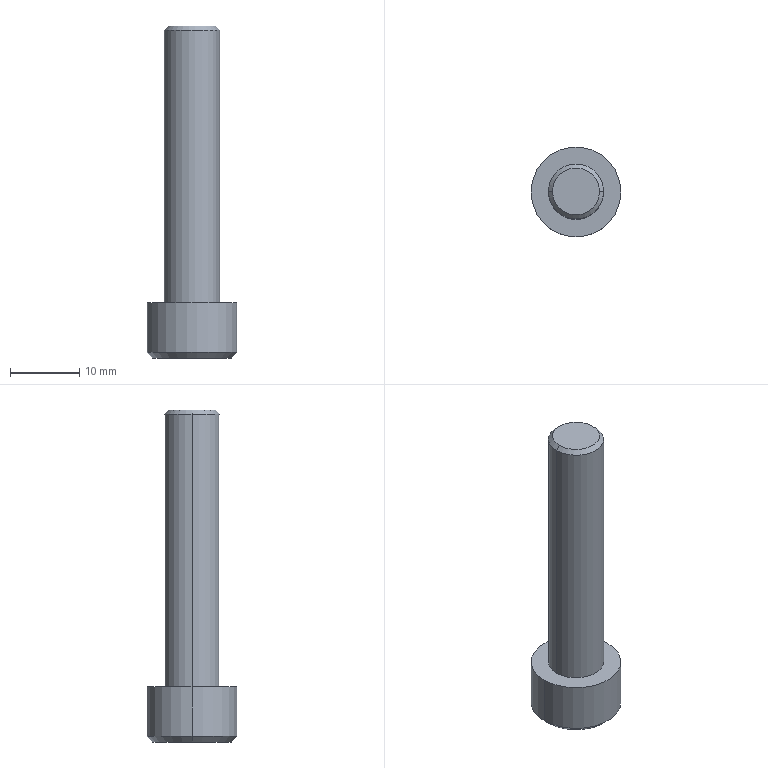Part | Creo | 1 solid | 18 faces | box 13 x 13 x 48 mm | volume 2906 mm3 | plane 10 | cylinder 4 | cone 4 | commonest cylinder face diameters 8 x2 13 x2
STEP:
#1=CARTESIAN_POINT('',(48.5,0.,-326.5));
#2=VERTEX_POINT('',#1);
#3=CARTESIAN_POINT('',(61.5,0.,-326.5));
#4=VERTEX_POINT('',#3);
#5=CARTESIAN_POINT('',(55.,0.,-326.5));
#6=DIRECTION('',(0.,0.,1.));
#7=DIRECTION('',(-1.,0.,0.));
#8=AXIS2_PLACEMENT_3D('',#5,#6,#7);
#9=CIRCLE('',#8,6.5);
#10=EDGE_CURVE('',#2,#4,#9,.T.);
#11=ORIENTED_EDGE('',*,*,#10,.F.);
#12=CARTESIAN_POINT('',(55.,0.,-326.5));
#13=DIRECTION('',(0.,0.,1.));
#14=DIRECTION('',(1.,0.,0.));
#15=AXIS2_PLACEMENT_3D('',#12,#13,#14);
#16=CIRCLE('',#15,6.5);
#17=EDGE_CURVE('',#4,#2,#16,.T.);
#18=ORIENTED_EDGE('',*,*,#17,.F.);
#19=EDGE_LOOP('',(#11,#18));
#20=FACE_OUTER_BOUND('',#19,.F.);
#21=CARTESIAN_POINT('',(59.,0.,-326.5));
#22=VERTEX_POINT('',#21);
#23=CARTESIAN_POINT('',(51.,0.,-326.5));
#24=VERTEX_POINT('',#23);
#25=CARTESIAN_POINT('',(55.,0.,-326.5));
#26=DIRECTION('',(0.,0.,-1.));
#27=DIRECTION('',(1.,0.,0.));
#28=AXIS2_PLACEMENT_3D('',#25,#26,#27);
#29=CIRCLE('',#28,4.);
#30=EDGE_CURVE('',#22,#24,#29,.T.);
#31=ORIENTED_EDGE('',*,*,#30,.F.);
#32=CARTESIAN_POINT('',(55.,0.,-326.5));
#33=DIRECTION('',(0.,0.,-1.));
#34=DIRECTION('',(-1.,0.,0.));
#35=AXIS2_PLACEMENT_3D('',#32,#33,#34);
#36=CIRCLE('',#35,4.);
#37=EDGE_CURVE('',#24,#22,#36,.T.);
#38=ORIENTED_EDGE('',*,*,#37,.F.);
#39=EDGE_LOOP('',(#31,#38));
#40=FACE_BOUND('',#39,.F.);
#41=CARTESIAN_POINT('',(55.,0.,-326.5));
#42=DIRECTION('',(0.,0.,1.));
#43=DIRECTION('',(1.,0.,0.));
#44=AXIS2_PLACEMENT_3D('',#41,#42,#43);
#45=PLANE('',#44);
#46=ADVANCED_FACE('',(#20,#40),#45,.T.);
#47=CARTESIAN_POINT('',(51.,0.,-287.1));
#48=VERTEX_POINT('',#47);
#49=CARTESIAN_POINT('',(59.,0.,-287.1));
#50=VERTEX_POINT('',#49);
#51=CARTESIAN_POINT('',(55.,0.,-287.1));
#52=DIRECTION('',(0.,0.,1.));
#53=DIRECTION('',(-1.,0.,0.));
#54=AXIS2_PLACEMENT_3D('',#51,#52,#53);
#55=CIRCLE('',#54,4.);
#56=EDGE_CURVE('',#48,#50,#55,.T.);
#57=ORIENTED_EDGE('',*,*,#56,.T.);
#58=CARTESIAN_POINT('',(59.,0.,-326.5));
#59=DIRECTION('',(0.,0.,1.));
#60=VECTOR('',#59,39.4);
#61=LINE('',#58,#60);
#62=EDGE_CURVE('',#22,#50,#61,.T.);
#63=ORIENTED_EDGE('',*,*,#62,.F.);
#64=ORIENTED_EDGE('',*,*,#30,.T.);
#65=CARTESIAN_POINT('',(51.,0.,-326.5));
#66=DIRECTION('',(0.,0.,1.));
#67=VECTOR('',#66,39.4);
#68=LINE('',#65,#67);
#69=EDGE_CURVE('',#24,#48,#68,.T.);
#70=ORIENTED_EDGE('',*,*,#69,.T.);
#71=EDGE_LOOP('',(#57,#63,#64,#70));
#72=FACE_OUTER_BOUND('',#71,.F.);
#73=CARTESIAN_POINT('',(55.,0.,-335.5));
#74=DIRECTION('',(0.,0.,1.));
#75=DIRECTION('',(1.,0.,0.));
#76=AXIS2_PLACEMENT_3D('',#73,#74,#75);
#77=CYLINDRICAL_SURFACE('',#76,4.);
#78=ADVANCED_FACE('',(#72),#77,.T.);
#79=CARTESIAN_POINT('',(51.6,0.,-286.5));
#80=VERTEX_POINT('',#79);
#81=CARTESIAN_POINT('',(58.4,0.,-286.5));
#82=VERTEX_POINT('',#81);
#83=CARTESIAN_POINT('',(55.,0.,-286.5));
#84=DIRECTION('',(0.,0.,1.));
#85=DIRECTION('',(-1.,0.,0.));
#86=AXIS2_PLACEMENT_3D('',#83,#84,#85);
#87=CIRCLE('',#86,3.4);
#88=EDGE_CURVE('',#80,#82,#87,.T.);
#89=ORIENTED_EDGE('',*,*,#88,.T.);
#90=CARTESIAN_POINT('',(58.4,0.,-286.5));
#91=DIRECTION('',(0.7071,0.,-0.7071));
#92=VECTOR('',#91,0.8485);
#93=LINE('',#90,#92);
#94=EDGE_CURVE('',#82,#50,#93,.T.);
#95=ORIENTED_EDGE('',*,*,#94,.T.);
#96=ORIENTED_EDGE('',*,*,#56,.F.);
#97=CARTESIAN_POINT('',(51.6,0.,-286.5));
#98=DIRECTION('',(-0.7071,0.,-0.7071));
#99=VECTOR('',#98,0.8485);
#100=LINE('',#97,#99);
#101=EDGE_CURVE('',#80,#48,#100,.T.);
#102=ORIENTED_EDGE('',*,*,#101,.F.);
#103=EDGE_LOOP('',(#89,#95,#96,#102));
#104=FACE_OUTER_BOUND('',#103,.F.);
#105=CARTESIAN_POINT('',(55.,0.,-286.8));
#106=DIRECTION('',(0.,0.,-1.));
#107=DIRECTION('',(-1.,0.,0.));
#108=AXIS2_PLACEMENT_3D('',#105,#106,#107);
#109=CONICAL_SURFACE('',#108,3.7,45.);
#110=ADVANCED_FACE('',(#104),#109,.T.);
#111=CARTESIAN_POINT('',(55.,0.,-286.5));
#112=DIRECTION('',(0.,0.,1.));
#113=DIRECTION('',(1.,0.,0.));
#114=AXIS2_PLACEMENT_3D('',#111,#112,#113);
#115=CIRCLE('',#114,3.4);
#116=EDGE_CURVE('',#82,#80,#115,.T.);
#117=ORIENTED_EDGE('',*,*,#116,.F.);
#118=ORIENTED_EDGE('',*,*,#88,.F.);
#119=EDGE_LOOP('',(#117,#118));
#120=FACE_OUTER_BOUND('',#119,.F.);
#121=CARTESIAN_POINT('',(55.,0.,-286.5));
#122=DIRECTION('',(0.,0.,1.));
#123=DIRECTION('',(1.,0.,0.));
#124=AXIS2_PLACEMENT_3D('',#121,#122,#123);
#125=PLANE('',#124);
#126=ADVANCED_FACE('',(#120),#125,.T.);
#127=ORIENTED_EDGE('',*,*,#116,.T.);
#128=ORIENTED_EDGE('',*,*,#101,.T.);
#129=CARTESIAN_POINT('',(55.,0.,-287.1));
#130=DIRECTION('',(0.,0.,1.));
#131=DIRECTION('',(1.,0.,0.));
#132=AXIS2_PLACEMENT_3D('',#129,#130,#131);
#133=CIRCLE('',#132,4.);
#134=EDGE_CURVE('',#50,#48,#133,.T.);
#135=ORIENTED_EDGE('',*,*,#134,.F.);
#136=ORIENTED_EDGE('',*,*,#94,.F.);
#137=EDGE_LOOP('',(#127,#128,#135,#136));
#138=FACE_OUTER_BOUND('',#137,.F.);
#139=CARTESIAN_POINT('',(55.,0.,-286.8));
#140=DIRECTION('',(0.,0.,-1.));
#141=DIRECTION('',(-1.,0.,0.));
#142=AXIS2_PLACEMENT_3D('',#139,#140,#141);
#143=CONICAL_SURFACE('',#142,3.7,45.);
#144=ADVANCED_FACE('',(#138),#143,.T.);
#145=ORIENTED_EDGE('',*,*,#134,.T.);
#146=ORIENTED_EDGE('',*,*,#69,.F.);
#147=ORIENTED_EDGE('',*,*,#37,.T.);
#148=ORIENTED_EDGE('',*,*,#62,.T.);
#149=EDGE_LOOP('',(#145,#146,#147,#148));
#150=FACE_OUTER_BOUND('',#149,.F.);
#151=CARTESIAN_POINT('',(55.,0.,-335.5));
#152=DIRECTION('',(0.,0.,1.));
#153=DIRECTION('',(1.,0.,0.));
#154=AXIS2_PLACEMENT_3D('',#151,#152,#153);
#155=CYLINDRICAL_SURFACE('',#154,4.);
#156=ADVANCED_FACE('',(#150),#155,.T.);
#157=CARTESIAN_POINT('',(61.5,0.,-333.7));
#158=VERTEX_POINT('',#157);
#159=CARTESIAN_POINT('',(48.5,0.,-333.7));
#160=VERTEX_POINT('',#159);
#161=CARTESIAN_POINT('',(55.,0.,-333.7));
#162=DIRECTION('',(0.,0.,-1.));
#163=DIRECTION('',(1.,0.,0.));
#164=AXIS2_PLACEMENT_3D('',#161,#162,#163);
#165=CIRCLE('',#164,6.5);
#166=EDGE_CURVE('',#158,#160,#165,.T.);
#167=ORIENTED_EDGE('',*,*,#166,.T.);
#168=CARTESIAN_POINT('',(48.5,0.,-333.7));
#169=DIRECTION('',(0.,0.,1.));
#170=VECTOR('',#169,7.2);
#171=LINE('',#168,#170);
#172=EDGE_CURVE('',#160,#2,#171,.T.);
#173=ORIENTED_EDGE('',*,*,#172,.T.);
#174=ORIENTED_EDGE('',*,*,#10,.T.);
#175=CARTESIAN_POINT('',(61.5,0.,-333.7));
#176=DIRECTION('',(0.,0.,1.));
#177=VECTOR('',#176,7.2);
#178=LINE('',#175,#177);
#179=EDGE_CURVE('',#158,#4,#178,.T.);
#180=ORIENTED_EDGE('',*,*,#179,.F.);
#181=EDGE_LOOP('',(#167,#173,#174,#180));
#182=FACE_OUTER_BOUND('',#181,.F.);
#183=CARTESIAN_POINT('',(55.,0.,-335.5));
#184=DIRECTION('',(0.,0.,1.));
#185=DIRECTION('',(1.,0.,0.));
#186=AXIS2_PLACEMENT_3D('',#183,#184,#185);
#187=CYLINDRICAL_SURFACE('',#186,6.5);
#188=ADVANCED_FACE('',(#182),#187,.T.);
#189=CARTESIAN_POINT('',(60.7,0.,-334.5));
#190=VERTEX_POINT('',#189);
#191=CARTESIAN_POINT('',(49.3,0.,-334.5));
#192=VERTEX_POINT('',#191);
#193=CARTESIAN_POINT('',(55.,0.,-334.5));
#194=DIRECTION('',(0.,0.,-1.));
#195=DIRECTION('',(1.,0.,0.));
#196=AXIS2_PLACEMENT_3D('',#193,#194,#195);
#197=CIRCLE('',#196,5.7);
#198=EDGE_CURVE('',#190,#192,#197,.T.);
#199=ORIENTED_EDGE('',*,*,#198,.T.);
#200=CARTESIAN_POINT('',(49.3,0.,-334.5));
#201=DIRECTION('',(-0.7071,0.,0.7071));
#202=VECTOR('',#201,1.131);
#203=LINE('',#200,#202);
#204=EDGE_CURVE('',#192,#160,#203,.T.);
#205=ORIENTED_EDGE('',*,*,#204,.T.);
#206=ORIENTED_EDGE('',*,*,#166,.F.);
#207=CARTESIAN_POINT('',(60.7,0.,-334.5));
#208=DIRECTION('',(0.7071,0.,0.7071));
#209=VECTOR('',#208,1.131);
#210=LINE('',#207,#209);
#211=EDGE_CURVE('',#190,#158,#210,.T.);
#212=ORIENTED_EDGE('',*,*,#211,.F.);
#213=EDGE_LOOP('',(#199,#205,#206,#212));
#214=FACE_OUTER_BOUND('',#213,.F.);
#215=CARTESIAN_POINT('',(55.,0.,-334.1));
#216=DIRECTION('',(0.,0.,1.));
#217=DIRECTION('',(1.,0.,0.));
#218=AXIS2_PLACEMENT_3D('',#215,#216,#217);
#219=CONICAL_SURFACE('',#218,6.1,45.);
#220=ADVANCED_FACE('',(#214),#219,.T.);
#221=ORIENTED_EDGE('',*,*,#198,.F.);
#222=CARTESIAN_POINT('',(55.,0.,-334.5));
#223=DIRECTION('',(0.,0.,-1.));
#224=DIRECTION('',(-1.,0.,0.));
#225=AXIS2_PLACEMENT_3D('',#222,#223,#224);
#226=CIRCLE('',#225,5.7);
#227=EDGE_CURVE('',#192,#190,#226,.T.);
#228=ORIENTED_EDGE('',*,*,#227,.F.);
#229=EDGE_LOOP('',(#221,#228));
#230=FACE_OUTER_BOUND('',#229,.F.);
#231=CARTESIAN_POINT('',(52.,-1.732,-334.5));
#232=VERTEX_POINT('',#231);
#233=CARTESIAN_POINT('',(55.,-3.464,-334.5));
#234=VERTEX_POINT('',#233);
#235=CARTESIAN_POINT('',(52.,-1.732,-334.5));
#236=DIRECTION('',(0.866,-0.5,0.));
#237=VECTOR('',#236,3.464);
#238=LINE('',#235,#237);
#239=EDGE_CURVE('',#232,#234,#238,.T.);
#240=ORIENTED_EDGE('',*,*,#239,.F.);
#241=CARTESIAN_POINT('',(52.,1.732,-334.5));
#242=VERTEX_POINT('',#241);
#243=CARTESIAN_POINT('',(52.,1.732,-334.5));
#244=DIRECTION('',(0.,-1.,0.));
#245=VECTOR('',#244,3.464);
#246=LINE('',#243,#245);
#247=EDGE_CURVE('',#242,#232,#246,.T.);
#248=ORIENTED_EDGE('',*,*,#247,.F.);
#249=CARTESIAN_POINT('',(55.,3.464,-334.5));
#250=VERTEX_POINT('',#249);
#251=CARTESIAN_POINT('',(55.,3.464,-334.5));
#252=DIRECTION('',(-0.866,-0.5,0.));
#253=VECTOR('',#252,3.464);
#254=LINE('',#251,#253);
#255=EDGE_CURVE('',#250,#242,#254,.T.);
#256=ORIENTED_EDGE('',*,*,#255,.F.);
#257=CARTESIAN_POINT('',(58.,1.732,-334.5));
#258=VERTEX_POINT('',#257);
#259=CARTESIAN_POINT('',(58.,1.732,-334.5));
#260=DIRECTION('',(-0.866,0.5,0.));
#261=VECTOR('',#260,3.464);
#262=LINE('',#259,#261);
#263=EDGE_CURVE('',#258,#250,#262,.T.);
#264=ORIENTED_EDGE('',*,*,#263,.F.);
#265=CARTESIAN_POINT('',(58.,-1.732,-334.5));
#266=VERTEX_POINT('',#265);
#267=CARTESIAN_POINT('',(58.,-1.732,-334.5));
#268=DIRECTION('',(0.,1.,0.));
#269=VECTOR('',#268,3.464);
#270=LINE('',#267,#269);
#271=EDGE_CURVE('',#266,#258,#270,.T.);
#272=ORIENTED_EDGE('',*,*,#271,.F.);
#273=CARTESIAN_POINT('',(55.,-3.464,-334.5));
#274=DIRECTION('',(0.866,0.5,0.));
#275=VECTOR('',#274,3.464);
#276=LINE('',#273,#275);
#277=EDGE_CURVE('',#234,#266,#276,.T.);
#278=ORIENTED_EDGE('',*,*,#277,.F.);
#279=EDGE_LOOP('',(#240,#248,#256,#264,#272,#278));
#280=FACE_BOUND('',#279,.F.);
#281=CARTESIAN_POINT('',(55.,0.,-334.5));
#282=DIRECTION('',(0.,0.,1.));
#283=DIRECTION('',(1.,0.,0.));
#284=AXIS2_PLACEMENT_3D('',#281,#282,#283);
#285=PLANE('',#284);
#286=ADVANCED_FACE('',(#230,#280),#285,.F.);
#287=ORIENTED_EDGE('',*,*,#227,.T.);
#288=ORIENTED_EDGE('',*,*,#211,.T.);
#289=CARTESIAN_POINT('',(55.,0.,-333.7));
#290=DIRECTION('',(0.,0.,-1.));
#291=DIRECTION('',(-1.,0.,0.));
#292=AXIS2_PLACEMENT_3D('',#289,#290,#291);
#293=CIRCLE('',#292,6.5);
#294=EDGE_CURVE('',#160,#158,#293,.T.);
#295=ORIENTED_EDGE('',*,*,#294,.F.);
#296=ORIENTED_EDGE('',*,*,#204,.F.);
#297=EDGE_LOOP('',(#287,#288,#295,#296));
#298=FACE_OUTER_BOUND('',#297,.F.);
#299=CARTESIAN_POINT('',(55.,0.,-334.1));
#300=DIRECTION('',(0.,0.,1.));
#301=DIRECTION('',(1.,0.,0.));
#302=AXIS2_PLACEMENT_3D('',#299,#300,#301);
#303=CONICAL_SURFACE('',#302,6.1,45.);
#304=ADVANCED_FACE('',(#298),#303,.T.);
#305=ORIENTED_EDGE('',*,*,#294,.T.);
#306=ORIENTED_EDGE('',*,*,#179,.T.);
#307=ORIENTED_EDGE('',*,*,#17,.T.);
#308=ORIENTED_EDGE('',*,*,#172,.F.);
#309=EDGE_LOOP('',(#305,#306,#307,#308));
#310=FACE_OUTER_BOUND('',#309,.F.);
#311=CARTESIAN_POINT('',(55.,0.,-335.5));
#312=DIRECTION('',(0.,0.,1.));
#313=DIRECTION('',(1.,0.,0.));
#314=AXIS2_PLACEMENT_3D('',#311,#312,#313);
#315=CYLINDRICAL_SURFACE('',#314,6.5);
#316=ADVANCED_FACE('',(#310),#315,.T.);
#317=ORIENTED_EDGE('',*,*,#239,.T.);
#318=CARTESIAN_POINT('',(55.,-3.464,-329.7));
#319=VERTEX_POINT('',#318);
#320=CARTESIAN_POINT('',(55.,-3.464,-334.5));
#321=DIRECTION('',(0.,0.,1.));
#322=VECTOR('',#321,4.8);
#323=LINE('',#320,#322);
#324=EDGE_CURVE('',#234,#319,#323,.T.);
#325=ORIENTED_EDGE('',*,*,#324,.T.);
#326=CARTESIAN_POINT('',(52.,-1.732,-329.7));
#327=VERTEX_POINT('',#326);
#328=CARTESIAN_POINT('',(55.,-3.464,-329.7));
#329=DIRECTION('',(-0.866,0.5,0.));
#330=VECTOR('',#329,3.464);
#331=LINE('',#328,#330);
#332=EDGE_CURVE('',#319,#327,#331,.T.);
#333=ORIENTED_EDGE('',*,*,#332,.T.);
#334=CARTESIAN_POINT('',(52.,-1.732,-334.5));
#335=DIRECTION('',(0.,0.,1.));
#336=VECTOR('',#335,4.8);
#337=LINE('',#334,#336);
#338=EDGE_CURVE('',#232,#327,#337,.T.);
#339=ORIENTED_EDGE('',*,*,#338,.F.);
#340=EDGE_LOOP('',(#317,#325,#333,#339));
#341=FACE_OUTER_BOUND('',#340,.F.);
#342=CARTESIAN_POINT('',(55.,-3.464,-329.7));
#343=DIRECTION('',(-0.5,-0.866,0.));
#344=DIRECTION('',(0.866,-0.5,0.));
#345=AXIS2_PLACEMENT_3D('',#342,#343,#344);
#346=PLANE('',#345);
#347=ADVANCED_FACE('',(#341),#346,.F.);
#348=ORIENTED_EDGE('',*,*,#277,.T.);
#349=CARTESIAN_POINT('',(58.,-1.732,-329.7));
#350=VERTEX_POINT('',#349);
#351=CARTESIAN_POINT('',(58.,-1.732,-334.5));
#352=DIRECTION('',(0.,0.,1.));
#353=VECTOR('',#352,4.8);
#354=LINE('',#351,#353);
#355=EDGE_CURVE('',#266,#350,#354,.T.);
#356=ORIENTED_EDGE('',*,*,#355,.T.);
#357=CARTESIAN_POINT('',(58.,-1.732,-329.7));
#358=DIRECTION('',(-0.866,-0.5,0.));
#359=VECTOR('',#358,3.464);
#360=LINE('',#357,#359);
#361=EDGE_CURVE('',#350,#319,#360,.T.);
#362=ORIENTED_EDGE('',*,*,#361,.T.);
#363=ORIENTED_EDGE('',*,*,#324,.F.);
#364=EDGE_LOOP('',(#348,#356,#362,#363));
#365=FACE_OUTER_BOUND('',#364,.F.);
#366=CARTESIAN_POINT('',(58.,-1.732,-329.7));
#367=DIRECTION('',(0.5,-0.866,0.));
#368=DIRECTION('',(0.866,0.5,0.));
#369=AXIS2_PLACEMENT_3D('',#366,#367,#368);
#370=PLANE('',#369);
#371=ADVANCED_FACE('',(#365),#370,.F.);
#372=ORIENTED_EDGE('',*,*,#271,.T.);
#373=CARTESIAN_POINT('',(58.,1.732,-329.7));
#374=VERTEX_POINT('',#373);
#375=CARTESIAN_POINT('',(58.,1.732,-334.5));
#376=DIRECTION('',(0.,0.,1.));
#377=VECTOR('',#376,4.8);
#378=LINE('',#375,#377);
#379=EDGE_CURVE('',#258,#374,#378,.T.);
#380=ORIENTED_EDGE('',*,*,#379,.T.);
#381=CARTESIAN_POINT('',(58.,-1.732,-329.7));
#382=DIRECTION('',(0.,1.,0.));
#383=VECTOR('',#382,3.464);
#384=LINE('',#381,#383);
#385=EDGE_CURVE('',#350,#374,#384,.T.);
#386=ORIENTED_EDGE('',*,*,#385,.F.);
#387=ORIENTED_EDGE('',*,*,#355,.F.);
#388=EDGE_LOOP('',(#372,#380,#386,#387));
#389=FACE_OUTER_BOUND('',#388,.F.);
#390=CARTESIAN_POINT('',(58.,1.732,-329.7));
#391=DIRECTION('',(1.,0.,0.));
#392=DIRECTION('',(0.,0.,-1.));
#393=AXIS2_PLACEMENT_3D('',#390,#391,#392);
#394=PLANE('',#393);
#395=ADVANCED_FACE('',(#389),#394,.F.);
#396=ORIENTED_EDGE('',*,*,#263,.T.);
#397=CARTESIAN_POINT('',(55.,3.464,-329.7));
#398=VERTEX_POINT('',#397);
#399=CARTESIAN_POINT('',(55.,3.464,-334.5));
#400=DIRECTION('',(0.,0.,1.));
#401=VECTOR('',#400,4.8);
#402=LINE('',#399,#401);
#403=EDGE_CURVE('',#250,#398,#402,.T.);
#404=ORIENTED_EDGE('',*,*,#403,.T.);
#405=CARTESIAN_POINT('',(55.,3.464,-329.7));
#406=DIRECTION('',(0.866,-0.5,0.));
#407=VECTOR('',#406,3.464);
#408=LINE('',#405,#407);
#409=EDGE_CURVE('',#398,#374,#408,.T.);
#410=ORIENTED_EDGE('',*,*,#409,.T.);
#411=ORIENTED_EDGE('',*,*,#379,.F.);
#412=EDGE_LOOP('',(#396,#404,#410,#411));
#413=FACE_OUTER_BOUND('',#412,.F.);
#414=CARTESIAN_POINT('',(55.,3.464,-329.7));
#415=DIRECTION('',(0.5,0.866,0.));
#416=DIRECTION('',(-0.866,0.5,0.));
#417=AXIS2_PLACEMENT_3D('',#414,#415,#416);
#418=PLANE('',#417);
#419=ADVANCED_FACE('',(#413),#418,.F.);
#420=ORIENTED_EDGE('',*,*,#255,.T.);
#421=CARTESIAN_POINT('',(52.,1.732,-329.7));
#422=VERTEX_POINT('',#421);
#423=CARTESIAN_POINT('',(52.,1.732,-334.5));
#424=DIRECTION('',(0.,0.,1.));
#425=VECTOR('',#424,4.8);
#426=LINE('',#423,#425);
#427=EDGE_CURVE('',#242,#422,#426,.T.);
#428=ORIENTED_EDGE('',*,*,#427,.T.);
#429=CARTESIAN_POINT('',(52.,1.732,-329.7));
#430=DIRECTION('',(0.866,0.5,0.));
#431=VECTOR('',#430,3.464);
#432=LINE('',#429,#431);
#433=EDGE_CURVE('',#422,#398,#432,.T.);
#434=ORIENTED_EDGE('',*,*,#433,.T.);
#435=ORIENTED_EDGE('',*,*,#403,.F.);
#436=EDGE_LOOP('',(#420,#428,#434,#435));
#437=FACE_OUTER_BOUND('',#436,.F.);
#438=CARTESIAN_POINT('',(52.,1.732,-329.7));
#439=DIRECTION('',(-0.5,0.866,0.));
#440=DIRECTION('',(-0.866,-0.5,0.));
#441=AXIS2_PLACEMENT_3D('',#438,#439,#440);
#442=PLANE('',#441);
#443=ADVANCED_FACE('',(#437),#442,.F.);
#444=ORIENTED_EDGE('',*,*,#247,.T.);
#445=ORIENTED_EDGE('',*,*,#338,.T.);
#446=CARTESIAN_POINT('',(52.,1.732,-329.7));
#447=DIRECTION('',(0.,-1.,0.));
#448=VECTOR('',#447,3.464);
#449=LINE('',#446,#448);
#450=EDGE_CURVE('',#422,#327,#449,.T.);
#451=ORIENTED_EDGE('',*,*,#450,.F.);
#452=ORIENTED_EDGE('',*,*,#427,.F.);
#453=EDGE_LOOP('',(#444,#445,#451,#452));
#454=FACE_OUTER_BOUND('',#453,.F.);
#455=CARTESIAN_POINT('',(52.,-1.732,-329.7));
#456=DIRECTION('',(-1.,0.,0.));
#457=DIRECTION('',(0.,0.,1.));
#458=AXIS2_PLACEMENT_3D('',#455,#456,#457);
#459=PLANE('',#458);
#460=ADVANCED_FACE('',(#454),#459,.F.);
#461=ORIENTED_EDGE('',*,*,#361,.F.);
#462=ORIENTED_EDGE('',*,*,#385,.T.);
#463=ORIENTED_EDGE('',*,*,#409,.F.);
#464=ORIENTED_EDGE('',*,*,#433,.F.);
#465=ORIENTED_EDGE('',*,*,#450,.T.);
#466=ORIENTED_EDGE('',*,*,#332,.F.);
#467=EDGE_LOOP('',(#461,#462,#463,#464,#465,#466));
#468=FACE_OUTER_BOUND('',#467,.F.);
#469=CARTESIAN_POINT('',(55.,-3.464,-329.7));
#470=DIRECTION('',(0.,0.,-1.));
#471=DIRECTION('',(-1.,0.,0.));
#472=AXIS2_PLACEMENT_3D('',#469,#470,#471);
#473=PLANE('',#472);
#474=ADVANCED_FACE('',(#468),#473,.T.);
#475=CLOSED_SHELL('',(#46,#78,#110,#126,#144,#156,#188,#220,#286,#304,#316,#347,#371,#395,#419,#443,#460,#474));
#476=MANIFOLD_SOLID_BREP('',#475);
#477=(LENGTH_UNIT()NAMED_UNIT(*)SI_UNIT(.MILLI.,.METRE.));
#478=UNCERTAINTY_MEASURE_WITH_UNIT(LENGTH_MEASURE(0.00514),#477,'','');
#479=(NAMED_UNIT(*)PLANE_ANGLE_UNIT()SI_UNIT($,.RADIAN.));
#480=PLANE_ANGLE_MEASURE_WITH_UNIT(PLANE_ANGLE_MEASURE(0.01745),#479);
#481=(CONVERSION_BASED_UNIT('DEGREE',#480)NAMED_UNIT(*)PLANE_ANGLE_UNIT());
#482=(NAMED_UNIT(*)SI_UNIT($,.STERADIAN.)SOLID_ANGLE_UNIT());
#483=(GEOMETRIC_REPRESENTATION_CONTEXT(3)GLOBAL_UNCERTAINTY_ASSIGNED_CONTEXT((#478))GLOBAL_UNIT_ASSIGNED_CONTEXT((#477,#481,#482))REPRESENTATION_CONTEXT('',''));
#484=ADVANCED_BREP_SHAPE_REPRESENTATION('',(#476),#483);